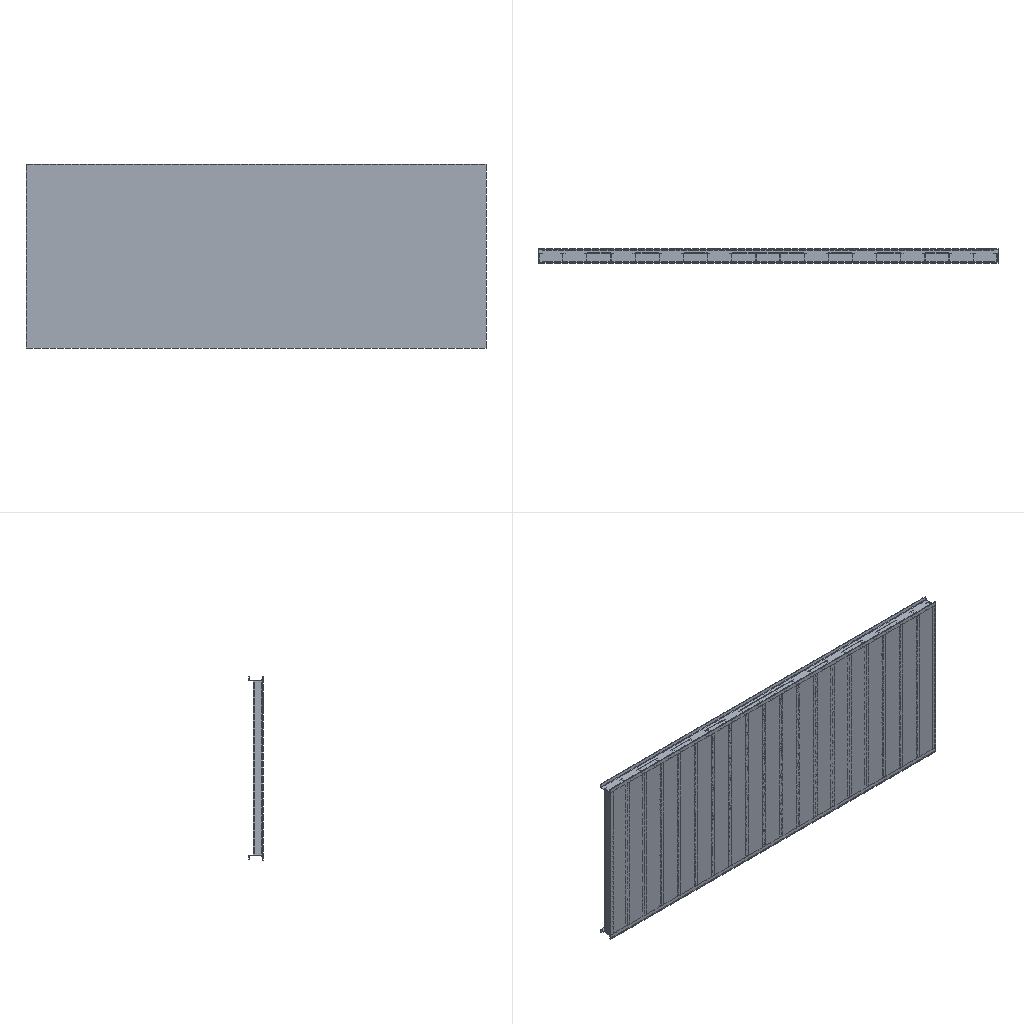Simulation study
Ansys APDL input file, long lists of numbers shortened:
/batch
/config,noeldb,1     ! force off writing results to database
*get,_wallstrt,active,,time,wall
! ANSYS input file written by Workbench version 2022 R1
! File used for geometry attach: F:\ansys（分析文件汇总)\结构件有限元分析qqww\fangan1_asm.STEP
/title,11--____ (C5)
! ****** Begin Custom Load Command Snippet ******
/COM, ACT Extensions:
/COM,     LSDYNA, 2021.1
/COM,
! ****** End   Custom Load Command Snippet ******
*DIM,_wb_ProjectScratch_dir,string,248
_wb_ProjectScratch_dir(1) = 'F:\ansys（分析文件汇总)\结构件有限元分析qqww\_ProjectScratch\Scr4449\'
*DIM,_wb_SolverFiles_dir,string,248
_wb_SolverFiles_dir(1) = 'F:\ansys（分析文件汇总)\结构件有限元分析qqww\11_files\dp0\SYS-1\MECH\'
*DIM,_wb_userfiles_dir,string,248
_wb_userfiles_dir(1) = 'F:\ansys（分析文件汇总)\结构件有限元分析qqww\11_files\user_files\'
/com,--- Data in consistent NMM units. See Solving Units in the help system for more information.
/units,MPA
/nopr
/wb,file,start              !  signify a WB generated input file
/prep7
! Turn off shape checking because checks already performed inside WB mesher.
! See help system for more information.
SHPP,OFF,,NOWARN
/nolist
etcon,set             ! allow ANSYS to choose best KEYOP's for 180x elements, resets any applicable keyopt to MAPDL defaults
/com,*********** Nodes for the whole assembly ***********
nblock,3,,220399
(1i9,3e20.9e3)
        1     2.625000000E+03     2.100000000E+02     1.577916667E+03
! (200362 more lines like these left out)
-1
/wb,elem,start            !  set before creation of elements
/com,*********** Elements for Body 1 "1040MUTAI-1|1040MUTAI-1[1]" ***********
et,1,187
eblock,19,solid,,24917
(19i9)
        1        1        1        1        0        0        0        0       10        0       73      867     7060     8664     7924    10636    48277    10639    10637
! (49833 more lines like these left out)
-1
/com,*********** Elements for Body 2 "1040MUTAI-2|1040MUTAI-2[1]" ***********
et,2,187
eblock,19,solid,,3615
(19i9)
        2        2        2        2        0        0        0        0       10        0    51415   103874   103912   103911   103950   106366   106528   106365   106368
! (7229 more lines like these left out)
-1
/com,*********** Elements for Body 3 "1040MUTAI-2|1040MUTAI-2[1][2]" ***********
et,3,187
eblock,19,solid,,3615
(19i9)
        3        3        3        3        0        0        0        0       10        0    44185    90138    90176    90175    90214    92630    92792    92629    92632
! (7229 more lines like these left out)
-1
/com,*********** Elements for Body 4 "1040MUTAI-2|1040MUTAI-2[1][3]" ***********
et,4,187
eblock,19,solid,,3615
(19i9)
        4        4        4        4        0        0        0        0       10        0    74973   153571   153609   153608   153647   156063   156225   156062   156065
! (7229 more lines like these left out)
-1
/com,*********** Elements for Body 5 "1040MUTAI-2|1040MUTAI-2[1][4]" ***********
et,5,187
eblock,19,solid,,3615
(19i9)
        5        5        5        5        0        0        0        0       10        0    36955    76402    76440    76439    76478    78894    79056    78893    78896
! (7229 more lines like these left out)
-1
! (27 more sections like these left out)
/wb,elem,end               !  done creating elements
/com,*********** Send User Defined Coordinate System(s) ***********
csys,0
toffst,273.15,  ! Temperature offset from absolute zero
/com,*********** Set Reference Temperature ***********
tref,22.
/wb,mat,start              !  starting to send materials
/com,*********** Send Materials ***********
Temperature = 'TEMP' ! Temperature
MP,DENS,1,7.85e-09,	! tonne mm^-3
MP,ALPX,1,1.2e-05,	! C^-1
MP,C,1,434000000,	! mm^2 s^-2 C^-1
MP,KXX,1,60.5,	! tonne mm s^-3 C^-1
MP,RSVX,1,0.00017,	! ohm mm
MP,EX,1,200000,	! tonne s^-2 mm^-1
MP,NUXY,1,0.3,
MP,MURX,1,10000,
Temperature = 'TEMP' ! Temperature
MP,DENS,2,7.85e-09,	! tonne mm^-3
MP,ALPX,2,1.2e-05,	! C^-1
MP,C,2,434000000,	! mm^2 s^-2 C^-1
MP,KXX,2,60.5,	! tonne mm s^-3 C^-1
MP,RSVX,2,0.00017,	! ohm mm
MP,EX,2,200000,	! tonne s^-2 mm^-1
MP,NUXY,2,0.3,
MP,MURX,2,10000,
Temperature = 'TEMP' ! Temperature
MP,DENS,3,7.85e-09,	! tonne mm^-3
MP,ALPX,3,1.2e-05,	! C^-1
MP,C,3,434000000,	! mm^2 s^-2 C^-1
MP,KXX,3,60.5,	! tonne mm s^-3 C^-1
MP,RSVX,3,0.00017,	! ohm mm
MP,EX,3,200000,	! tonne s^-2 mm^-1
MP,NUXY,3,0.3,
MP,MURX,3,10000,
Temperature = 'TEMP' ! Temperature
MP,DENS,4,7.85e-09,	! tonne mm^-3
MP,ALPX,4,1.2e-05,	! C^-1
MP,C,4,434000000,	! mm^2 s^-2 C^-1
MP,KXX,4,60.5,	! tonne mm s^-3 C^-1
MP,RSVX,4,0.00017,	! ohm mm
MP,EX,4,200000,	! tonne s^-2 mm^-1
MP,NUXY,4,0.3,
MP,MURX,4,10000,
Temperature = 'TEMP' ! Temperature
MP,DENS,5,7.85e-09,	! tonne mm^-3
MP,ALPX,5,1.2e-05,	! C^-1
MP,C,5,434000000,	! mm^2 s^-2 C^-1
MP,KXX,5,60.5,	! tonne mm s^-3 C^-1
MP,RSVX,5,0.00017,	! ohm mm
MP,EX,5,200000,	! tonne s^-2 mm^-1
MP,NUXY,5,0.3,
MP,MURX,5,10000,
Temperature = 'TEMP' ! Temperature
MP,DENS,6,7.85e-09,	! tonne mm^-3
MP,ALPX,6,1.2e-05,	! C^-1
MP,C,6,434000000,	! mm^2 s^-2 C^-1
MP,KXX,6,60.5,	! tonne mm s^-3 C^-1
MP,RSVX,6,0.00017,	! ohm mm
MP,EX,6,200000,	! tonne s^-2 mm^-1
MP,NUXY,6,0.3,
MP,MURX,6,10000,
Temperature = 'TEMP' ! Temperature
MP,DENS,7,7.85e-09,	! tonne mm^-3
MP,ALPX,7,1.2e-05,	! C^-1
MP,C,7,434000000,	! mm^2 s^-2 C^-1
MP,KXX,7,60.5,	! tonne mm s^-3 C^-1
MP,RSVX,7,0.00017,	! ohm mm
MP,EX,7,200000,	! tonne s^-2 mm^-1
MP,NUXY,7,0.3,
MP,MURX,7,10000,
Temperature = 'TEMP' ! Temperature
MP,DENS,8,7.85e-09,	! tonne mm^-3
MP,ALPX,8,1.2e-05,	! C^-1
MP,C,8,434000000,	! mm^2 s^-2 C^-1
MP,KXX,8,60.5,	! tonne mm s^-3 C^-1
MP,RSVX,8,0.00017,	! ohm mm
MP,EX,8,200000,	! tonne s^-2 mm^-1
MP,NUXY,8,0.3,
MP,MURX,8,10000,
Temperature = 'TEMP' ! Temperature
MP,DENS,9,7.85e-09,	! tonne mm^-3
MP,ALPX,9,1.2e-05,	! C^-1
MP,C,9,434000000,	! mm^2 s^-2 C^-1
MP,KXX,9,60.5,	! tonne mm s^-3 C^-1
MP,RSVX,9,0.00017,	! ohm mm
MP,EX,9,200000,	! tonne s^-2 mm^-1
! (209 more lines like these left out)
/wb,mat,end                !  done sending materials
!************************* Model Summary ********************
!1040MUTAI-1|1040MUTAI-1[1],	Q235,	matid,	1
!1040MUTAI-2|1040MUTAI-2[1],	Q235,	matid,	2
!1040MUTAI-2|1040MUTAI-2[1][2],	Q235,	matid,	3
! (31 more lines like these left out)
*get,_xmin,node,,mnloc,x
*get,_ymin,node,,mnloc,y
*get,_zmin,node,,mnloc,z
*get,_xmax,node,,mxloc,x
*get,_ymax,node,,mxloc,y
*get,_zmax,node,,mxloc,z
_ASMDIAG=(_xmax-_xmin)*(_xmax-_xmin)+(_ymax-_ymin)*(_ymax-_ymin)+(_zmax-_zmin)*(_zmax-_zmin)
_ASMDIAG=SQRT(_ASMDIAG)
/wb,contact,start          !  starting to send contact
/com,*********** Create Contact "接触区域" ***********
/com,            Real Constant Set For Above Contact Is 34 & 33
*set,tid,34
*set,cid,33
r,tid
r,cid
et,tid,170
et,cid,174
eblock,10,,,243
(15i9)
   160448       34       34       34        0     7637     9258     8085     8085    49690    50477     8085    49689
! (242 more lines like these left out)
-1
eblock,10,,,243
(15i9)
   160691       33       33       33        0     7637     9258     8085     8085    49690    50477     8085    49689
! (242 more lines like these left out)
-1
eblock,10,,,152
(15i9)
   160934       33       34       33        0   104734   103843   104757   104757   106123   106124   104757   110526
! (151 more lines like these left out)
-1
eblock,10,,,152
(15i9)
   161086       34       33       34        0   104734   103843   104757   104757   106123   106124   104757   110526
! (151 more lines like these left out)
-1
keyo,cid,8,2               ! auto create asymmetric contact (from Program Controlled setting)
keyo,cid,10,0              ! adjust contact stiffness each NR iteration (from Program Controlled setting)
keyo,cid,12,5              ! bonded always
keyo,cid,18,1              ! small sliding turned on by application
keyo,cid,2,0               ! augmented Lagrange (from Program Controlled setting)
keyo,cid,4,0               ! on Gauss point (from Program Controlled setting)
keyo,cid,9,1               ! ignore initial gaps/penetration
keyo,cid,7,0               ! No Prediction
rmod,tid,3,10.      ! FKN
rmod,tid,5,0.       ! ICONT
rmod,tid,6,0.       ! PINB
rmod,tid,10,0.      ! CNOF
rmod,tid,12,0.      ! FKT
rmod,tid,36,92      ! WB DSID
rmod,cid,3,10.      ! FKN
rmod,cid,5,0.       ! ICONT
rmod,cid,6,0.       ! PINB
rmod,cid,10,0.      ! CNOF
rmod,cid,12,0.      ! FKT
rmod,cid,36,92      ! WB DSID
/com,*********** Create Contact "接触区域 2" ***********
/com,            Real Constant Set For Above Contact Is 36 & 35
*set,tid,36
*set,cid,35
r,tid
r,cid
et,tid,170
et,cid,174
eblock,10,,,253
(15i9)
   161238       36       36       36        0     7714     8203     9171     9171    49855    50645     9171    49856
! (252 more lines like these left out)
-1
eblock,10,,,253
(15i9)
   161491       35       35       35        0     7714     8203     9171     9171    49855    50645     9171    49856
! (252 more lines like these left out)
-1
eblock,10,,,152
(15i9)
   161744       35       36       35        0    90998    90107    91021    91021    92387    92388    91021    96790
! (151 more lines like these left out)
-1
eblock,10,,,152
(15i9)
   161896       36       35       36        0    90998    90107    91021    91021    92387    92388    91021    96790
! (151 more lines like these left out)
-1
keyo,cid,8,2               ! auto create asymmetric contact (from Program Controlled setting)
keyo,cid,10,0              ! adjust contact stiffness each NR iteration (from Program Controlled setting)
keyo,cid,12,5              ! bonded always
keyo,cid,18,1              ! small sliding turned on by application
keyo,cid,2,0               ! augmented Lagrange (from Program Controlled setting)
keyo,cid,4,0               ! on Gauss point (from Program Controlled setting)
keyo,cid,9,1               ! ignore initial gaps/penetration
keyo,cid,7,0               ! No Prediction
rmod,tid,3,10.      ! FKN
rmod,tid,5,0.       ! ICONT
rmod,tid,6,0.       ! PINB
rmod,tid,10,0.      ! CNOF
rmod,tid,12,0.      ! FKT
rmod,tid,36,95      ! WB DSID
rmod,cid,3,10.      ! FKN
rmod,cid,5,0.       ! ICONT
rmod,cid,6,0.       ! PINB
rmod,cid,10,0.      ! CNOF
rmod,cid,12,0.      ! FKT
rmod,cid,36,95      ! WB DSID
/com,*********** Create Contact "接触区域 3" ***********
/com,            Real Constant Set For Above Contact Is 38 & 37
*set,tid,38
*set,cid,37
r,tid
r,cid
et,tid,170
et,cid,174
eblock,10,,,241
(15i9)
   162048       38       38       38        0     5780     6567     8300     8300    42461    46551     8300    42466
! (240 more lines like these left out)
-1
eblock,10,,,241
(15i9)
   162289       37       37       37        0     5780     6567     8300     8300    42461    46551     8300    42466
! (240 more lines like these left out)
-1
eblock,10,,,152
(15i9)
   162530       37       38       37        0   154431   153540   154454   154454   155820   155821   154454   160223
! (151 more lines like these left out)
-1
eblock,10,,,152
(15i9)
   162682       38       37       38        0   154431   153540   154454   154454   155820   155821   154454   160223
! (151 more lines like these left out)
-1
keyo,cid,8,2               ! auto create asymmetric contact (from Program Controlled setting)
keyo,cid,10,0              ! adjust contact stiffness each NR iteration (from Program Controlled setting)
keyo,cid,12,5              ! bonded always
keyo,cid,18,1              ! small sliding turned on by application
keyo,cid,2,0               ! augmented Lagrange (from Program Controlled setting)
keyo,cid,4,0               ! on Gauss point (from Program Controlled setting)
keyo,cid,9,1               ! ignore initial gaps/penetration
keyo,cid,7,0               ! No Prediction
rmod,tid,3,10.      ! FKN
rmod,tid,5,0.       ! ICONT
rmod,tid,6,0.       ! PINB
rmod,tid,10,0.      ! CNOF
rmod,tid,12,0.      ! FKT
rmod,tid,36,98      ! WB DSID
rmod,cid,3,10.      ! FKN
rmod,cid,5,0.       ! ICONT
rmod,cid,6,0.       ! PINB
rmod,cid,10,0.      ! CNOF
rmod,cid,12,0.      ! FKT
rmod,cid,36,98      ! WB DSID
/com,*********** Create Contact "接触区域 4" ***********
/com,            Real Constant Set For Above Contact Is 40 & 39
*set,tid,40
*set,cid,39
r,tid
r,cid
et,tid,170
et,cid,174
eblock,10,,,239
(15i9)
   162834       40       40       40        0     6948     8003     8359     8359    47927    50331     8359    47928
! (238 more lines like these left out)
-1
eblock,10,,,239
(15i9)
   163073       39       39       39        0     6948     8003     8359     8359    47927    50331     8359    47928
! (238 more lines like these left out)
-1
eblock,10,,,152
(15i9)
   163312       39       40       39        0    77262    76371    77285    77285    78651    78652    77285    83054
! (151 more lines like these left out)
-1
eblock,10,,,152
(15i9)
   163464       40       39       40        0    77262    76371    77285    77285    78651    78652    77285    83054
! (151 more lines like these left out)
-1
keyo,cid,8,2               ! auto create asymmetric contact (from Program Controlled setting)
keyo,cid,10,0              ! adjust contact stiffness each NR iteration (from Program Controlled setting)
keyo,cid,12,5              ! bonded always
keyo,cid,18,1              ! small sliding turned on by application
keyo,cid,2,0               ! augmented Lagrange (from Program Controlled setting)
keyo,cid,4,0               ! on Gauss point (from Program Controlled setting)
keyo,cid,9,1               ! ignore initial gaps/penetration
keyo,cid,7,0               ! No Prediction
rmod,tid,3,10.      ! FKN
rmod,tid,5,0.       ! ICONT
rmod,tid,6,0.       ! PINB
rmod,tid,10,0.      ! CNOF
rmod,tid,12,0.      ! FKT
rmod,tid,36,101     ! WB DSID
rmod,cid,3,10.      ! FKN
rmod,cid,5,0.       ! ICONT
rmod,cid,6,0.       ! PINB
rmod,cid,10,0.      ! CNOF
rmod,cid,12,0.      ! FKT
rmod,cid,36,101     ! WB DSID
/com,*********** Create Contact "接触区域 5" ***********
/com,            Real Constant Set For Above Contact Is 42 & 41
*set,tid,42
*set,cid,41
r,tid
r,cid
et,tid,170
et,cid,174
eblock,10,,,275
(15i9)
   163616       42       42       42        0     5562     6938     6899     6899    41099    47770     6899    41098
! (274 more lines like these left out)
-1
eblock,10,,,275
(15i9)
   163891       41       41       41        0     5562     6938     6899     6899    41099    47770     6899    41098
! (274 more lines like these left out)
-1
eblock,10,,,152
(15i9)
   164166       41       42       41        0   161299   160408   161322   161322   162688   162689   161322   167091
! (151 more lines like these left out)
-1
eblock,10,,,152
(15i9)
   164318       42       41       42        0   161299   160408   161322   161322   162688   162689   161322   167091
! (151 more lines like these left out)
-1
keyo,cid,8,2               ! auto create asymmetric contact (from Program Controlled setting)
keyo,cid,10,0              ! adjust contact stiffness each NR iteration (from Program Controlled setting)
keyo,cid,12,5              ! bonded always
keyo,cid,18,1              ! small sliding turned on by application
keyo,cid,2,0               ! augmented Lagrange (from Program Controlled setting)
keyo,cid,4,0               ! on Gauss point (from Program Controlled setting)
keyo,cid,9,1               ! ignore initial gaps/penetration
keyo,cid,7,0               ! No Prediction
rmod,tid,3,10.      ! FKN
rmod,tid,5,0.       ! ICONT
rmod,tid,6,0.       ! PINB
rmod,tid,10,0.      ! CNOF
rmod,tid,12,0.      ! FKT
rmod,tid,36,104     ! WB DSID
rmod,cid,3,10.      ! FKN
rmod,cid,5,0.       ! ICONT
rmod,cid,6,0.       ! PINB
rmod,cid,10,0.      ! CNOF
rmod,cid,12,0.      ! FKT
rmod,cid,36,104     ! WB DSID
! (95 more sections like these left out)
/wb,contact,end            !  done creating contacts
/golist
/wb,load,start             !  starting to send loads
/com,*********** Fixed Supports ***********
CMBLOCK,_FIXEDSU,NODE,     1206
(8i10)
     51432     51433     52140     52141     52142     52143     52144     52145
! (150 more lines like these left out)
cmsel,s,_FIXEDSU
d,all,all
nsel,all
/com,*********** Define Force Using Surface Effect Elements ***********
local,12,0,0.,0.,0.,0.,0.,0.
csys,0
et,233,154
eblock,10,,,918
(15i9)
   187396      233      233      233       12      866     2873      867      867    10620    10631      867    10619
! (917 more lines like these left out)
-1
esel,s,type,,233
keyop,233,2,1                ! Apply load in local coordinate system
keyop,233,7,1                ! Use original area so load is constant in large deformation
esel,all
/com,*********** Define Force Using Surface Effect Elements ***********
local,13,0,0.,0.,0.,0.,0.,0.
csys,0
et,234,154
eblock,10,,,216
(15i9)
   188314      234      234      234       13      732      733     5284     5284     9395     9408     5284     9398
! (215 more lines like these left out)
-1
esel,s,type,,234
keyop,234,2,1                ! Apply load in local coordinate system
keyop,234,7,1                ! Use original area so load is constant in large deformation
esel,all
/gst,on,on
fini
*get,_numnode,node,0,count
*get,_numelem,elem,0,count
*get, _MAXELEMNUM, elem, 0, NUM, MAX
*get, _MAXNODENUM, node, 0, NUM, MAX
*get, _MAXELEMTYPE, etyp, 0, NUM, MAX
*get, _MAXREALCONST, real, 0, NUM, MAX
/go
/wb,load,end               !  done creating loads
/com,--- Number of total nodes = %_numnode%
/com,--- Number of contact elements = 28082
/com,--- Number of spring elements = 0
/com,--- Number of bearing elements = 0
/com,--- Number of solid elements = 99715
/com,--- Number of condensed parts = 0
/com,--- Number of total elements = %_numelem%
*get,_wallbsol,active,,time,wall
/com,****************************************************************************
/com,*************************    SOLUTION       ********************************
/com,****************************************************************************
/solu
antype,0                   ! static analysis
_thickRatio=0.0625  ! Ratio of thick parts in the model
eqsl,sparse,,,,,1
cntr,print,1               ! print out contact info and also make no initial contact an error
dmpoption,emat,no             ! Don't combine emat file for DANSYS
dmpoption,esav,no             ! Don't combine esav file for DANSYS
nldiag,cont,iter           ! print out contact info each equilibrium iteration
rescontrol,,none                 ! Do not keep any restart files
/com,****************************************************
/com,******************* SOLVE FOR LS 1 OF 1 ****************
esel,s,type,,233
nsle
sfe,all,1,pres,1,0.
sfe,all,2,pres,1,6.55725419664068e-002
sfe,all,3,pres,1,0.
esel,s,type,,234
nsle
sfe,all,1,pres,1,0.
sfe,all,2,pres,1,0.2083
sfe,all,3,pres,1,0.
nsel,all
esel,all
acel,0.,0.,9806.65
/nopr
/gopr
nsub,1,1,1
time,1.
outres,erase
outres,all,none
outres,nsol,all,
outres,rsol,all
outres,eangl,all
outres,etmp,all
outres,veng,all
outres,strs,all,
outres,epel,all,
outres,eppl,all,
outres,cont,all,
! *********** WB SOLVE COMMAND ***********
! check interactive state
*get,ANSINTER_,active,,int
*if,ANSINTER_,ne,0,then
/eof
*endif
solve
/com *************** Write FE CONNECTORS *********
CEWRITE,file,ce,,INTE
/com,****************************************************
/com,*************** FINISHED SOLVE FOR LS 1 *************
*get,_wallasol,active,,time,wall
/nopr
*get,_numnode,node,0,count
*get,_numelem,elem,0,count
*get, _MAXELEMNUM, elem, 0, NUM, MAX
*get, _MAXNODENUM, node, 0, NUM, MAX,,,INTERNAL
*get, _MAXELEMTYPE, etyp, 0, NUM, MAX
*get, _MAXREALCONST, real, 0, NUM, MAX
/gopr
/post1
xmlo,ENCODING,ISO-8859-1
xmlo,parm
/xml,parm,xml
fini
/gopr
*get,_walldone,active,,time,wall
_preptime=(_wallbsol-_wallstrt)*3600
_solvtime=(_wallasol-_wallbsol)*3600
_posttime=(_walldone-_wallasol)*3600
_totaltim=(_walldone-_wallstrt)*3600
*get,_dlbratio,active,0,solu,dlbr
*get,_combtime,active,0,solu,comb
*get,_ssmode,active,0,solu,ssmm
*get,_ndofs,active,0,solu,ndof
*get,_sol_end_time,active,0,set,time
*if,_sol_end_time,eq,1.,then
/fclean				!clean distributed files
*endif
/com,--- Total number of nodes = %_numnode%
/com,--- Total number of elements = %_numelem%
/com,--- Element load balance ratio = %_dlbratio%
/com,--- Time to combine distributed files = %_combtime%
/com,--- Sparse memory mode = %_ssmode%
/com,--- Number of DOF = %_ndofs%
/wb,file,end               ! done with WB generated input